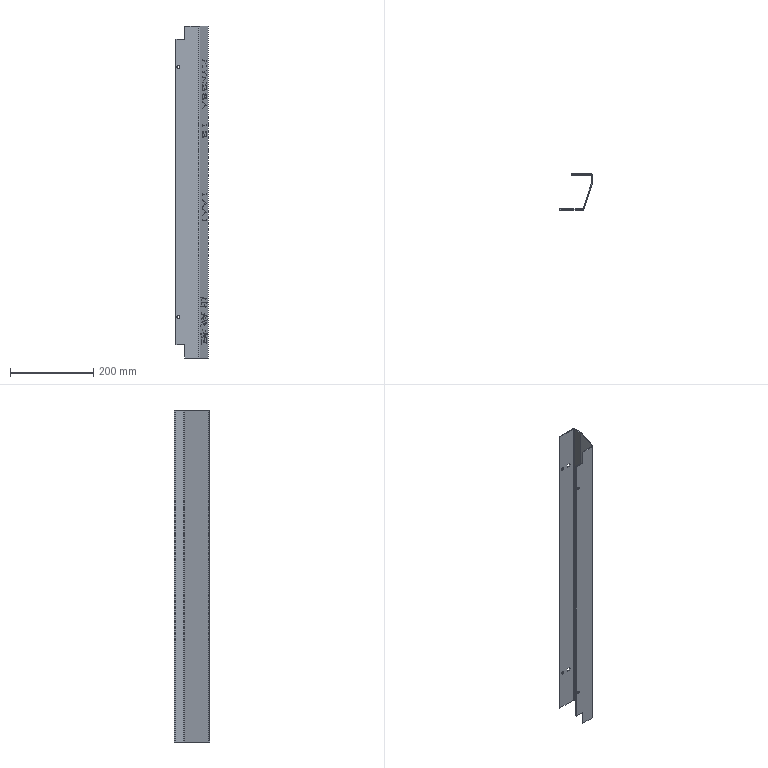Part | STEP file | Top flange (flat door) AA | 1 solid | 559 faces | box 77.333 x 86 x 798 mm | volume 299938 mm3 | plane 355 | spline 190 | cylinder 14 | commonest cylinder face diameters 7 x11 3 x3